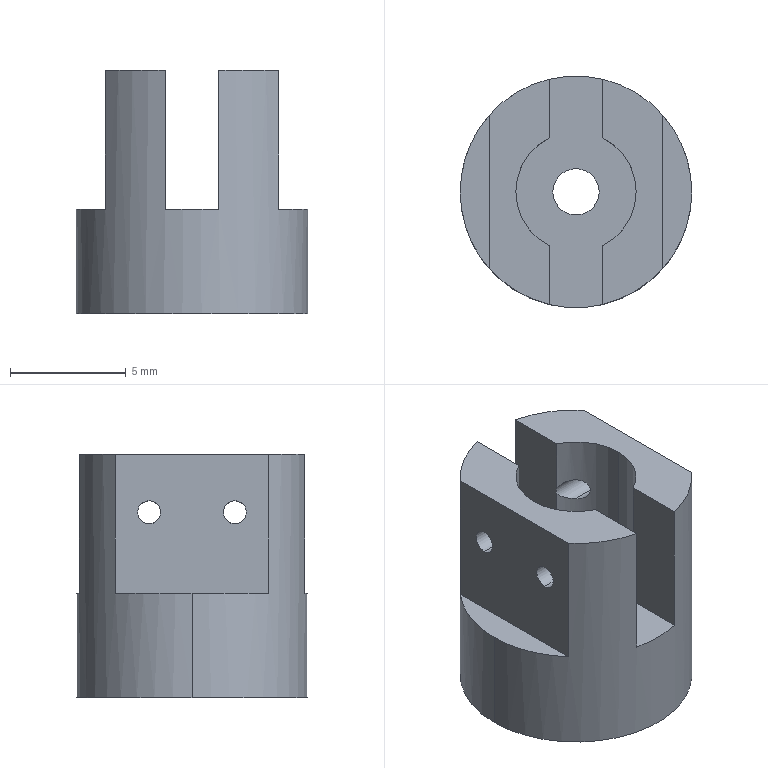Part | SolidWorks | features ICE 6, Extrusion 1 | 1 solid | 30 faces | box 10 x 10 x 10.5 mm | volume 483.8 mm3 | cylinder 17 | plane 13 | commonest cylinder face diameters 1 x8 5.2 x3 2 x2 5 x2 10 x2
STEP:
#1=CARTESIAN_POINT('',(3.75,1.85,7.5));
#2=VERTEX_POINT('',#1);
#3=CARTESIAN_POINT('',(3.75,1.85,8.5));
#4=VERTEX_POINT('',#3);
#5=CARTESIAN_POINT('',(3.75,1.85,8.));
#6=DIRECTION('',(-1.,0.,0.));
#7=DIRECTION('',(0.,0.,1.));
#8=AXIS2_PLACEMENT_3D('',#5,#6,#7);
#9=CIRCLE('',#8,0.5);
#10=EDGE_CURVE('',#2,#4,#9,.T.);
#11=ORIENTED_EDGE('',*,*,#10,.F.);
#12=CARTESIAN_POINT('',(1.827,1.85,7.5));
#13=VERTEX_POINT('',#12);
#14=CARTESIAN_POINT('',(5.,1.85,7.5));
#15=DIRECTION('',(-1.,0.,0.));
#16=VECTOR('',#15,1000.);
#17=LINE('',#14,#16);
#18=EDGE_CURVE('',#2,#13,#17,.T.);
#19=ORIENTED_EDGE('',*,*,#18,.T.);
#20=CARTESIAN_POINT('',(1.827,1.85,8.5));
#21=VERTEX_POINT('',#20);
#22=CARTESIAN_POINT('',(1.827,1.85,8.5));
#23=CARTESIAN_POINT('',(1.934,1.744,8.5));
#24=CARTESIAN_POINT('',(2.032,1.626,8.466));
#25=CARTESIAN_POINT('',(2.142,1.475,8.338));
#26=CARTESIAN_POINT('',(2.171,1.431,8.282));
#27=CARTESIAN_POINT('',(2.211,1.368,8.152));
#28=CARTESIAN_POINT('',(2.222,1.35,8.077));
#29=CARTESIAN_POINT('',(2.222,1.35,7.926));
#30=CARTESIAN_POINT('',(2.212,1.368,7.85));
#31=CARTESIAN_POINT('',(2.172,1.43,7.719));
#32=CARTESIAN_POINT('',(2.142,1.475,7.663));
#33=CARTESIAN_POINT('',(2.069,1.576,7.577));
#34=CARTESIAN_POINT('',(2.026,1.631,7.547));
#35=CARTESIAN_POINT('',(1.931,1.742,7.508));
#36=CARTESIAN_POINT('',(1.881,1.797,7.5));
#37=CARTESIAN_POINT('',(1.827,1.85,7.5));
#38=B_SPLINE_CURVE_WITH_KNOTS('',3,(#22,#23,#24,#25,#26,#27,#28,#29,#30,#31,#32,#33,#34,#35,#36,#37),.UNSPECIFIED.,.F.,.F.,(4,2,2,2,2,2,2,4),(0.0009388,0.001388,0.001612,0.001836,0.002061,0.002285,0.00251,0.002734),.UNSPECIFIED.);
#39=EDGE_CURVE('',#21,#13,#38,.T.);
#40=ORIENTED_EDGE('',*,*,#39,.F.);
#41=CARTESIAN_POINT('',(5.,1.85,8.5));
#42=DIRECTION('',(-1.,0.,0.));
#43=VECTOR('',#42,1000.);
#44=LINE('',#41,#43);
#45=EDGE_CURVE('',#4,#21,#44,.T.);
#46=ORIENTED_EDGE('',*,*,#45,.F.);
#47=EDGE_LOOP('',(#11,#19,#40,#46));
#48=FACE_OUTER_BOUND('',#47,.T.);
#49=CARTESIAN_POINT('',(5.,1.85,8.));
#50=DIRECTION('',(-1.,0.,0.));
#51=DIRECTION('',(0.,0.,1.));
#52=AXIS2_PLACEMENT_3D('',#49,#50,#51);
#53=CYLINDRICAL_SURFACE('',#52,0.5);
#54=ADVANCED_FACE('',(#48),#53,.F.);
#55=CARTESIAN_POINT('',(3.75,-1.85,7.5));
#56=VERTEX_POINT('',#55);
#57=CARTESIAN_POINT('',(3.75,-1.85,8.5));
#58=VERTEX_POINT('',#57);
#59=CARTESIAN_POINT('',(3.75,-1.85,8.));
#60=DIRECTION('',(-1.,0.,0.));
#61=DIRECTION('',(0.,0.,1.));
#62=AXIS2_PLACEMENT_3D('',#59,#60,#61);
#63=CIRCLE('',#62,0.5);
#64=EDGE_CURVE('',#56,#58,#63,.T.);
#65=ORIENTED_EDGE('',*,*,#64,.F.);
#66=CARTESIAN_POINT('',(1.827,-1.85,7.5));
#67=VERTEX_POINT('',#66);
#68=CARTESIAN_POINT('',(5.,-1.85,7.5));
#69=DIRECTION('',(-1.,0.,0.));
#70=VECTOR('',#69,1000.);
#71=LINE('',#68,#70);
#72=EDGE_CURVE('',#56,#67,#71,.T.);
#73=ORIENTED_EDGE('',*,*,#72,.T.);
#74=CARTESIAN_POINT('',(1.15,-2.332,7.866));
#75=VERTEX_POINT('',#74);
#76=CARTESIAN_POINT('',(1.15,-2.332,7.866));
#77=CARTESIAN_POINT('',(1.188,-2.313,7.799));
#78=CARTESIAN_POINT('',(1.242,-2.285,7.747));
#79=CARTESIAN_POINT('',(1.355,-2.22,7.659));
#80=CARTESIAN_POINT('',(1.414,-2.183,7.624));
#81=CARTESIAN_POINT('',(1.594,-2.059,7.535));
#82=CARTESIAN_POINT('',(1.715,-1.96,7.5));
#83=CARTESIAN_POINT('',(1.827,-1.85,7.5));
#84=B_SPLINE_CURVE_WITH_KNOTS('',3,(#76,#77,#78,#79,#80,#81,#82,#83),.UNSPECIFIED.,.F.,.F.,(4,2,2,4),(0.,0.0002347,0.0004694,0.0009388),.UNSPECIFIED.);
#85=EDGE_CURVE('',#75,#67,#84,.T.);
#86=ORIENTED_EDGE('',*,*,#85,.F.);
#87=CARTESIAN_POINT('',(1.15,-2.332,8.134));
#88=VERTEX_POINT('',#87);
#89=CARTESIAN_POINT('',(1.15,-1.85,8.));
#90=DIRECTION('',(1.,0.,0.));
#91=DIRECTION('',(0.,0.,-1.));
#92=AXIS2_PLACEMENT_3D('',#89,#90,#91);
#93=CIRCLE('',#92,0.5);
#94=EDGE_CURVE('',#88,#75,#93,.T.);
#95=ORIENTED_EDGE('',*,*,#94,.F.);
#96=CARTESIAN_POINT('',(1.827,-1.85,8.5));
#97=VERTEX_POINT('',#96);
#98=CARTESIAN_POINT('',(1.827,-1.85,8.5));
#99=CARTESIAN_POINT('',(1.714,-1.961,8.5));
#100=CARTESIAN_POINT('',(1.593,-2.06,8.465));
#101=CARTESIAN_POINT('',(1.414,-2.183,8.376));
#102=CARTESIAN_POINT('',(1.355,-2.22,8.341));
#103=CARTESIAN_POINT('',(1.242,-2.285,8.253));
#104=CARTESIAN_POINT('',(1.188,-2.313,8.201));
#105=CARTESIAN_POINT('',(1.15,-2.332,8.134));
#106=B_SPLINE_CURVE_WITH_KNOTS('',3,(#98,#99,#100,#101,#102,#103,#104,#105),.UNSPECIFIED.,.F.,.F.,(4,2,2,4),(0.002734,0.003203,0.003438,0.003673),.UNSPECIFIED.);
#107=EDGE_CURVE('',#97,#88,#106,.T.);
#108=ORIENTED_EDGE('',*,*,#107,.F.);
#109=CARTESIAN_POINT('',(5.,-1.85,8.5));
#110=DIRECTION('',(-1.,0.,0.));
#111=VECTOR('',#110,1000.);
#112=LINE('',#109,#111);
#113=EDGE_CURVE('',#58,#97,#112,.T.);
#114=ORIENTED_EDGE('',*,*,#113,.F.);
#115=EDGE_LOOP('',(#65,#73,#86,#95,#108,#114));
#116=FACE_OUTER_BOUND('',#115,.T.);
#117=CARTESIAN_POINT('',(5.,-1.85,8.));
#118=DIRECTION('',(-1.,0.,0.));
#119=DIRECTION('',(0.,0.,1.));
#120=AXIS2_PLACEMENT_3D('',#117,#118,#119);
#121=CYLINDRICAL_SURFACE('',#120,0.5);
#122=ADVANCED_FACE('',(#116),#121,.F.);
#123=CARTESIAN_POINT('',(-1.827,1.85,7.5));
#124=VERTEX_POINT('',#123);
#125=CARTESIAN_POINT('',(-1.827,1.85,8.5));
#126=VERTEX_POINT('',#125);
#127=CARTESIAN_POINT('',(-1.827,1.85,7.5));
#128=CARTESIAN_POINT('',(-1.934,1.744,7.5));
#129=CARTESIAN_POINT('',(-2.032,1.626,7.534));
#130=CARTESIAN_POINT('',(-2.142,1.475,7.662));
#131=CARTESIAN_POINT('',(-2.171,1.431,7.718));
#132=CARTESIAN_POINT('',(-2.211,1.368,7.848));
#133=CARTESIAN_POINT('',(-2.222,1.35,7.923));
#134=CARTESIAN_POINT('',(-2.222,1.35,8.074));
#135=CARTESIAN_POINT('',(-2.212,1.368,8.15));
#136=CARTESIAN_POINT('',(-2.172,1.43,8.281));
#137=CARTESIAN_POINT('',(-2.142,1.475,8.337));
#138=CARTESIAN_POINT('',(-2.069,1.576,8.423));
#139=CARTESIAN_POINT('',(-2.026,1.631,8.453));
#140=CARTESIAN_POINT('',(-1.931,1.742,8.492));
#141=CARTESIAN_POINT('',(-1.881,1.797,8.5));
#142=CARTESIAN_POINT('',(-1.827,1.85,8.5));
#143=B_SPLINE_CURVE_WITH_KNOTS('',3,(#127,#128,#129,#130,#131,#132,#133,#134,#135,#136,#137,#138,#139,#140,#141,#142),.UNSPECIFIED.,.F.,.F.,(4,2,2,2,2,2,2,4),(0.0009388,0.001388,0.001612,0.001836,0.002061,0.002285,0.00251,0.002734),.UNSPECIFIED.);
#144=EDGE_CURVE('',#124,#126,#143,.T.);
#145=ORIENTED_EDGE('',*,*,#144,.F.);
#146=CARTESIAN_POINT('',(-3.75,1.85,7.5));
#147=VERTEX_POINT('',#146);
#148=CARTESIAN_POINT('',(5.,1.85,7.5));
#149=DIRECTION('',(-1.,0.,0.));
#150=VECTOR('',#149,1000.);
#151=LINE('',#148,#150);
#152=EDGE_CURVE('',#124,#147,#151,.T.);
#153=ORIENTED_EDGE('',*,*,#152,.T.);
#154=CARTESIAN_POINT('',(-3.75,1.85,8.5));
#155=VERTEX_POINT('',#154);
#156=CARTESIAN_POINT('',(-3.75,1.85,8.));
#157=DIRECTION('',(-1.,0.,0.));
#158=DIRECTION('',(0.,0.,1.));
#159=AXIS2_PLACEMENT_3D('',#156,#157,#158);
#160=CIRCLE('',#159,0.5);
#161=EDGE_CURVE('',#147,#155,#160,.T.);
#162=ORIENTED_EDGE('',*,*,#161,.T.);
#163=CARTESIAN_POINT('',(5.,1.85,8.5));
#164=DIRECTION('',(-1.,0.,0.));
#165=VECTOR('',#164,1000.);
#166=LINE('',#163,#165);
#167=EDGE_CURVE('',#126,#155,#166,.T.);
#168=ORIENTED_EDGE('',*,*,#167,.F.);
#169=EDGE_LOOP('',(#145,#153,#162,#168));
#170=FACE_OUTER_BOUND('',#169,.T.);
#171=CARTESIAN_POINT('',(5.,1.85,8.));
#172=DIRECTION('',(-1.,0.,0.));
#173=DIRECTION('',(0.,0.,1.));
#174=AXIS2_PLACEMENT_3D('',#171,#172,#173);
#175=CYLINDRICAL_SURFACE('',#174,0.5);
#176=ADVANCED_FACE('',(#170),#175,.F.);
#177=CARTESIAN_POINT('',(-1.827,-1.85,7.5));
#178=VERTEX_POINT('',#177);
#179=CARTESIAN_POINT('',(-1.15,-2.332,7.866));
#180=VERTEX_POINT('',#179);
#181=CARTESIAN_POINT('',(-1.827,-1.85,7.5));
#182=CARTESIAN_POINT('',(-1.714,-1.961,7.5));
#183=CARTESIAN_POINT('',(-1.593,-2.06,7.535));
#184=CARTESIAN_POINT('',(-1.414,-2.183,7.624));
#185=CARTESIAN_POINT('',(-1.355,-2.22,7.659));
#186=CARTESIAN_POINT('',(-1.242,-2.285,7.747));
#187=CARTESIAN_POINT('',(-1.188,-2.313,7.799));
#188=CARTESIAN_POINT('',(-1.15,-2.332,7.866));
#189=B_SPLINE_CURVE_WITH_KNOTS('',3,(#181,#182,#183,#184,#185,#186,#187,#188),.UNSPECIFIED.,.F.,.F.,(4,2,2,4),(0.002734,0.003203,0.003438,0.003673),.UNSPECIFIED.);
#190=EDGE_CURVE('',#178,#180,#189,.T.);
#191=ORIENTED_EDGE('',*,*,#190,.F.);
#192=CARTESIAN_POINT('',(-3.75,-1.85,7.5));
#193=VERTEX_POINT('',#192);
#194=CARTESIAN_POINT('',(5.,-1.85,7.5));
#195=DIRECTION('',(-1.,0.,0.));
#196=VECTOR('',#195,1000.);
#197=LINE('',#194,#196);
#198=EDGE_CURVE('',#178,#193,#197,.T.);
#199=ORIENTED_EDGE('',*,*,#198,.T.);
#200=CARTESIAN_POINT('',(-3.75,-1.85,8.5));
#201=VERTEX_POINT('',#200);
#202=CARTESIAN_POINT('',(-3.75,-1.85,8.));
#203=DIRECTION('',(-1.,0.,0.));
#204=DIRECTION('',(0.,0.,1.));
#205=AXIS2_PLACEMENT_3D('',#202,#203,#204);
#206=CIRCLE('',#205,0.5);
#207=EDGE_CURVE('',#193,#201,#206,.T.);
#208=ORIENTED_EDGE('',*,*,#207,.T.);
#209=CARTESIAN_POINT('',(-1.827,-1.85,8.5));
#210=VERTEX_POINT('',#209);
#211=CARTESIAN_POINT('',(5.,-1.85,8.5));
#212=DIRECTION('',(-1.,0.,0.));
#213=VECTOR('',#212,1000.);
#214=LINE('',#211,#213);
#215=EDGE_CURVE('',#210,#201,#214,.T.);
#216=ORIENTED_EDGE('',*,*,#215,.F.);
#217=CARTESIAN_POINT('',(-1.15,-2.332,8.134));
#218=VERTEX_POINT('',#217);
#219=CARTESIAN_POINT('',(-1.15,-2.332,8.134));
#220=CARTESIAN_POINT('',(-1.188,-2.313,8.201));
#221=CARTESIAN_POINT('',(-1.242,-2.285,8.253));
#222=CARTESIAN_POINT('',(-1.355,-2.22,8.341));
#223=CARTESIAN_POINT('',(-1.414,-2.183,8.376));
#224=CARTESIAN_POINT('',(-1.594,-2.059,8.465));
#225=CARTESIAN_POINT('',(-1.715,-1.96,8.5));
#226=CARTESIAN_POINT('',(-1.827,-1.85,8.5));
#227=B_SPLINE_CURVE_WITH_KNOTS('',3,(#219,#220,#221,#222,#223,#224,#225,#226),.UNSPECIFIED.,.F.,.F.,(4,2,2,4),(0.,0.0002347,0.0004694,0.0009388),.UNSPECIFIED.);
#228=EDGE_CURVE('',#218,#210,#227,.T.);
#229=ORIENTED_EDGE('',*,*,#228,.F.);
#230=CARTESIAN_POINT('',(-1.15,-1.85,8.));
#231=DIRECTION('',(-1.,0.,0.));
#232=DIRECTION('',(0.,0.,1.));
#233=AXIS2_PLACEMENT_3D('',#230,#231,#232);
#234=CIRCLE('',#233,0.5);
#235=EDGE_CURVE('',#180,#218,#234,.T.);
#236=ORIENTED_EDGE('',*,*,#235,.F.);
#237=EDGE_LOOP('',(#191,#199,#208,#216,#229,#236));
#238=FACE_OUTER_BOUND('',#237,.T.);
#239=CARTESIAN_POINT('',(5.,-1.85,8.));
#240=DIRECTION('',(-1.,0.,0.));
#241=DIRECTION('',(0.,0.,1.));
#242=AXIS2_PLACEMENT_3D('',#239,#240,#241);
#243=CYLINDRICAL_SURFACE('',#242,0.5);
#244=ADVANCED_FACE('',(#238),#243,.F.);
#245=CARTESIAN_POINT('',(2.6,0.,4.5));
#246=VERTEX_POINT('',#245);
#247=CARTESIAN_POINT('',(1.15,2.332,4.5));
#248=VERTEX_POINT('',#247);
#249=CARTESIAN_POINT('',(0.,0.,4.5));
#250=DIRECTION('',(0.,0.,1.));
#251=DIRECTION('',(-1.,0.,0.));
#252=AXIS2_PLACEMENT_3D('',#249,#250,#251);
#253=CIRCLE('',#252,2.6);
#254=EDGE_CURVE('',#246,#248,#253,.T.);
#255=ORIENTED_EDGE('',*,*,#254,.F.);
#256=CARTESIAN_POINT('',(2.6,0.,10.5));
#257=VERTEX_POINT('',#256);
#258=CARTESIAN_POINT('',(2.6,0.,-2.854));
#259=DIRECTION('',(0.,0.,1.));
#260=VECTOR('',#259,1000.);
#261=LINE('',#258,#260);
#262=EDGE_CURVE('',#246,#257,#261,.T.);
#263=ORIENTED_EDGE('',*,*,#262,.T.);
#264=CARTESIAN_POINT('',(1.15,2.332,10.5));
#265=VERTEX_POINT('',#264);
#266=CARTESIAN_POINT('',(0.,0.,10.5));
#267=DIRECTION('',(0.,0.,1.));
#268=DIRECTION('',(1.,0.,0.));
#269=AXIS2_PLACEMENT_3D('',#266,#267,#268);
#270=CIRCLE('',#269,2.6);
#271=EDGE_CURVE('',#257,#265,#270,.T.);
#272=ORIENTED_EDGE('',*,*,#271,.T.);
#273=CARTESIAN_POINT('',(1.15,2.332,8.134));
#274=VERTEX_POINT('',#273);
#275=CARTESIAN_POINT('',(1.15,2.332,-2.854));
#276=DIRECTION('',(0.,0.,1.));
#277=VECTOR('',#276,1000.);
#278=LINE('',#275,#277);
#279=EDGE_CURVE('',#274,#265,#278,.T.);
#280=ORIENTED_EDGE('',*,*,#279,.F.);
#281=CARTESIAN_POINT('',(1.15,2.332,8.134));
#282=CARTESIAN_POINT('',(1.188,2.313,8.201));
#283=CARTESIAN_POINT('',(1.242,2.285,8.253));
#284=CARTESIAN_POINT('',(1.355,2.22,8.341));
#285=CARTESIAN_POINT('',(1.414,2.183,8.376));
#286=CARTESIAN_POINT('',(1.594,2.059,8.465));
#287=CARTESIAN_POINT('',(1.715,1.96,8.5));
#288=CARTESIAN_POINT('',(1.827,1.85,8.5));
#289=B_SPLINE_CURVE_WITH_KNOTS('',3,(#281,#282,#283,#284,#285,#286,#287,#288),.UNSPECIFIED.,.F.,.F.,(4,2,2,4),(0.,0.0002347,0.0004694,0.0009388),.UNSPECIFIED.);
#290=EDGE_CURVE('',#274,#21,#289,.T.);
#291=ORIENTED_EDGE('',*,*,#290,.T.);
#292=ORIENTED_EDGE('',*,*,#39,.T.);
#293=CARTESIAN_POINT('',(1.15,2.332,7.866));
#294=VERTEX_POINT('',#293);
#295=CARTESIAN_POINT('',(1.827,1.85,7.5));
#296=CARTESIAN_POINT('',(1.714,1.961,7.5));
#297=CARTESIAN_POINT('',(1.593,2.06,7.535));
#298=CARTESIAN_POINT('',(1.414,2.183,7.624));
#299=CARTESIAN_POINT('',(1.355,2.22,7.659));
#300=CARTESIAN_POINT('',(1.242,2.285,7.747));
#301=CARTESIAN_POINT('',(1.188,2.313,7.799));
#302=CARTESIAN_POINT('',(1.15,2.332,7.866));
#303=B_SPLINE_CURVE_WITH_KNOTS('',3,(#295,#296,#297,#298,#299,#300,#301,#302),.UNSPECIFIED.,.F.,.F.,(4,2,2,4),(0.002734,0.003203,0.003438,0.003673),.UNSPECIFIED.);
#304=EDGE_CURVE('',#13,#294,#303,.T.);
#305=ORIENTED_EDGE('',*,*,#304,.T.);
#306=CARTESIAN_POINT('',(1.15,2.332,-2.854));
#307=DIRECTION('',(0.,0.,1.));
#308=VECTOR('',#307,1000.);
#309=LINE('',#306,#308);
#310=EDGE_CURVE('',#248,#294,#309,.T.);
#311=ORIENTED_EDGE('',*,*,#310,.F.);
#312=EDGE_LOOP('',(#255,#263,#272,#280,#291,#292,#305,#311));
#313=FACE_OUTER_BOUND('',#312,.T.);
#314=CARTESIAN_POINT('',(0.,0.,-2.854));
#315=DIRECTION('',(0.,0.,1.));
#316=DIRECTION('',(1.,0.,0.));
#317=AXIS2_PLACEMENT_3D('',#314,#315,#316);
#318=CYLINDRICAL_SURFACE('',#317,2.6);
#319=ADVANCED_FACE('',(#313),#318,.F.);
#320=CARTESIAN_POINT('',(-1.,0.,4.5));
#321=VERTEX_POINT('',#320);
#322=CARTESIAN_POINT('',(1.,0.,4.5));
#323=VERTEX_POINT('',#322);
#324=CARTESIAN_POINT('',(0.,0.,4.5));
#325=DIRECTION('',(0.,0.,1.));
#326=DIRECTION('',(-1.,0.,0.));
#327=AXIS2_PLACEMENT_3D('',#324,#325,#326);
#328=CIRCLE('',#327,1.);
#329=EDGE_CURVE('',#321,#323,#328,.T.);
#330=ORIENTED_EDGE('',*,*,#329,.T.);
#331=CARTESIAN_POINT('',(1.,0.,3.5));
#332=VERTEX_POINT('',#331);
#333=CARTESIAN_POINT('',(1.,0.,10.5));
#334=DIRECTION('',(0.,0.,-1.));
#335=VECTOR('',#334,1000.);
#336=LINE('',#333,#335);
#337=EDGE_CURVE('',#323,#332,#336,.T.);
#338=ORIENTED_EDGE('',*,*,#337,.T.);
#339=CARTESIAN_POINT('',(-1.,0.,3.5));
#340=VERTEX_POINT('',#339);
#341=CARTESIAN_POINT('',(0.,0.,3.5));
#342=DIRECTION('',(0.,0.,-1.));
#343=DIRECTION('',(-1.,0.,0.));
#344=AXIS2_PLACEMENT_3D('',#341,#342,#343);
#345=CIRCLE('',#344,1.);
#346=EDGE_CURVE('',#332,#340,#345,.T.);
#347=ORIENTED_EDGE('',*,*,#346,.T.);
#348=CARTESIAN_POINT('',(-1.,0.,10.5));
#349=DIRECTION('',(0.,0.,-1.));
#350=VECTOR('',#349,1000.);
#351=LINE('',#348,#350);
#352=EDGE_CURVE('',#321,#340,#351,.T.);
#353=ORIENTED_EDGE('',*,*,#352,.F.);
#354=EDGE_LOOP('',(#330,#338,#347,#353));
#355=FACE_OUTER_BOUND('',#354,.T.);
#356=CARTESIAN_POINT('',(0.,0.,10.5));
#357=DIRECTION('',(0.,0.,-1.));
#358=DIRECTION('',(-1.,0.,0.));
#359=AXIS2_PLACEMENT_3D('',#356,#357,#358);
#360=CYLINDRICAL_SURFACE('',#359,1.);
#361=ADVANCED_FACE('',(#355),#360,.F.);
#362=CARTESIAN_POINT('',(2.5,0.,3.5));
#363=VERTEX_POINT('',#362);
#364=CARTESIAN_POINT('',(-2.5,0.,3.5));
#365=VERTEX_POINT('',#364);
#366=CARTESIAN_POINT('',(0.,0.,3.5));
#367=DIRECTION('',(0.,0.,-1.));
#368=DIRECTION('',(-1.,0.,0.));
#369=AXIS2_PLACEMENT_3D('',#366,#367,#368);
#370=CIRCLE('',#369,2.5);
#371=EDGE_CURVE('',#363,#365,#370,.T.);
#372=ORIENTED_EDGE('',*,*,#371,.F.);
#373=CARTESIAN_POINT('',(2.5,0.,0.));
#374=VERTEX_POINT('',#373);
#375=CARTESIAN_POINT('',(2.5,0.,3.5));
#376=DIRECTION('',(0.,0.,-1.));
#377=VECTOR('',#376,1000.);
#378=LINE('',#375,#377);
#379=EDGE_CURVE('',#363,#374,#378,.T.);
#380=ORIENTED_EDGE('',*,*,#379,.T.);
#381=CARTESIAN_POINT('',(-2.5,0.,0.));
#382=VERTEX_POINT('',#381);
#383=CARTESIAN_POINT('',(0.,0.,0.));
#384=DIRECTION('',(0.,0.,-1.));
#385=DIRECTION('',(-1.,0.,0.));
#386=AXIS2_PLACEMENT_3D('',#383,#384,#385);
#387=CIRCLE('',#386,2.5);
#388=EDGE_CURVE('',#374,#382,#387,.T.);
#389=ORIENTED_EDGE('',*,*,#388,.T.);
#390=CARTESIAN_POINT('',(-2.5,0.,3.5));
#391=DIRECTION('',(0.,0.,-1.));
#392=VECTOR('',#391,1000.);
#393=LINE('',#390,#392);
#394=EDGE_CURVE('',#365,#382,#393,.T.);
#395=ORIENTED_EDGE('',*,*,#394,.F.);
#396=EDGE_LOOP('',(#372,#380,#389,#395));
#397=FACE_OUTER_BOUND('',#396,.T.);
#398=CARTESIAN_POINT('',(0.,0.,3.5));
#399=DIRECTION('',(0.,0.,-1.));
#400=DIRECTION('',(-1.,0.,0.));
#401=AXIS2_PLACEMENT_3D('',#398,#399,#400);
#402=CYLINDRICAL_SURFACE('',#401,2.5);
#403=ADVANCED_FACE('',(#397),#402,.F.);
#404=CARTESIAN_POINT('',(3.75,3.307,4.5));
#405=VERTEX_POINT('',#404);
#406=CARTESIAN_POINT('',(5.,0.,4.5));
#407=VERTEX_POINT('',#406);
#408=CARTESIAN_POINT('',(0.,0.,4.5));
#409=DIRECTION('',(0.,0.,-1.));
#410=DIRECTION('',(-1.,0.,0.));
#411=AXIS2_PLACEMENT_3D('',#408,#409,#410);
#412=CIRCLE('',#411,5.);
#413=EDGE_CURVE('',#405,#407,#412,.T.);
#414=ORIENTED_EDGE('',*,*,#413,.T.);
#415=CARTESIAN_POINT('',(5.,0.,0.));
#416=VERTEX_POINT('',#415);
#417=CARTESIAN_POINT('',(5.,0.,10.5));
#418=DIRECTION('',(0.,0.,-1.));
#419=VECTOR('',#418,1000.);
#420=LINE('',#417,#419);
#421=EDGE_CURVE('',#407,#416,#420,.T.);
#422=ORIENTED_EDGE('',*,*,#421,.T.);
#423=CARTESIAN_POINT('',(-5.,0.,0.));
#424=VERTEX_POINT('',#423);
#425=CARTESIAN_POINT('',(0.,0.,0.));
#426=DIRECTION('',(0.,0.,1.));
#427=DIRECTION('',(1.,0.,0.));
#428=AXIS2_PLACEMENT_3D('',#425,#426,#427);
#429=CIRCLE('',#428,5.);
#430=EDGE_CURVE('',#416,#424,#429,.T.);
#431=ORIENTED_EDGE('',*,*,#430,.T.);
#432=CARTESIAN_POINT('',(-5.,0.,4.5));
#433=VERTEX_POINT('',#432);
#434=CARTESIAN_POINT('',(-5.,0.,10.5));
#435=DIRECTION('',(0.,0.,-1.));
#436=VECTOR('',#435,1000.);
#437=LINE('',#434,#436);
#438=EDGE_CURVE('',#433,#424,#437,.T.);
#439=ORIENTED_EDGE('',*,*,#438,.F.);
#440=CARTESIAN_POINT('',(-3.75,3.307,4.5));
#441=VERTEX_POINT('',#440);
#442=CARTESIAN_POINT('',(0.,0.,4.5));
#443=DIRECTION('',(0.,0.,-1.));
#444=DIRECTION('',(-1.,0.,0.));
#445=AXIS2_PLACEMENT_3D('',#442,#443,#444);
#446=CIRCLE('',#445,5.);
#447=EDGE_CURVE('',#433,#441,#446,.T.);
#448=ORIENTED_EDGE('',*,*,#447,.T.);
#449=CARTESIAN_POINT('',(-3.75,3.307,10.5));
#450=VERTEX_POINT('',#449);
#451=CARTESIAN_POINT('',(-3.75,3.307,10.5));
#452=DIRECTION('',(0.,0.,1.));
#453=VECTOR('',#452,1000.);
#454=LINE('',#451,#453);
#455=EDGE_CURVE('',#441,#450,#454,.T.);
#456=ORIENTED_EDGE('',*,*,#455,.T.);
#457=CARTESIAN_POINT('',(-1.15,4.866,10.5));
#458=VERTEX_POINT('',#457);
#459=CARTESIAN_POINT('',(0.,0.,10.5));
#460=DIRECTION('',(0.,0.,1.));
#461=DIRECTION('',(1.,0.,0.));
#462=AXIS2_PLACEMENT_3D('',#459,#460,#461);
#463=CIRCLE('',#462,5.);
#464=EDGE_CURVE('',#458,#450,#463,.T.);
#465=ORIENTED_EDGE('',*,*,#464,.F.);
#466=CARTESIAN_POINT('',(-1.15,4.866,4.5));
#467=VERTEX_POINT('',#466);
#468=CARTESIAN_POINT('',(-1.15,4.866,10.5));
#469=DIRECTION('',(0.,0.,-1.));
#470=VECTOR('',#469,1000.);
#471=LINE('',#468,#470);
#472=EDGE_CURVE('',#458,#467,#471,.T.);
#473=ORIENTED_EDGE('',*,*,#472,.T.);
#474=CARTESIAN_POINT('',(1.15,4.866,4.5));
#475=VERTEX_POINT('',#474);
#476=CARTESIAN_POINT('',(0.,0.,4.5));
#477=DIRECTION('',(0.,0.,-1.));
#478=DIRECTION('',(-1.,0.,0.));
#479=AXIS2_PLACEMENT_3D('',#476,#477,#478);
#480=CIRCLE('',#479,5.);
#481=EDGE_CURVE('',#467,#475,#480,.T.);
#482=ORIENTED_EDGE('',*,*,#481,.T.);
#483=CARTESIAN_POINT('',(1.15,4.866,10.5));
#484=VERTEX_POINT('',#483);
#485=CARTESIAN_POINT('',(1.15,4.866,10.5));
#486=DIRECTION('',(0.,0.,1.));
#487=VECTOR('',#486,1000.);
#488=LINE('',#485,#487);
#489=EDGE_CURVE('',#475,#484,#488,.T.);
#490=ORIENTED_EDGE('',*,*,#489,.T.);
#491=CARTESIAN_POINT('',(3.75,3.307,10.5));
#492=VERTEX_POINT('',#491);
#493=CARTESIAN_POINT('',(0.,0.,10.5));
#494=DIRECTION('',(0.,0.,1.));
#495=DIRECTION('',(1.,0.,0.));
#496=AXIS2_PLACEMENT_3D('',#493,#494,#495);
#497=CIRCLE('',#496,5.);
#498=EDGE_CURVE('',#492,#484,#497,.T.);
#499=ORIENTED_EDGE('',*,*,#498,.F.);
#500=CARTESIAN_POINT('',(3.75,3.307,10.5));
#501=DIRECTION('',(0.,0.,-1.));
#502=VECTOR('',#501,1000.);
#503=LINE('',#500,#502);
#504=EDGE_CURVE('',#492,#405,#503,.T.);
#505=ORIENTED_EDGE('',*,*,#504,.T.);
#506=EDGE_LOOP('',(#414,#422,#431,#439,#448,#456,#465,#473,#482,#490,#499,#505));
#507=FACE_OUTER_BOUND('',#506,.T.);
#508=CARTESIAN_POINT('',(0.,0.,10.5));
#509=DIRECTION('',(0.,0.,-1.));
#510=DIRECTION('',(-1.,0.,0.));
#511=AXIS2_PLACEMENT_3D('',#508,#509,#510);
#512=CYLINDRICAL_SURFACE('',#511,5.);
#513=ADVANCED_FACE('',(#507),#512,.T.);
#514=CARTESIAN_POINT('',(-1.15,-2.332,4.5));
#515=VERTEX_POINT('',#514);
#516=CARTESIAN_POINT('',(-1.15,-2.332,-2.854));
#517=DIRECTION('',(0.,0.,1.));
#518=VECTOR('',#517,1000.);
#519=LINE('',#516,#518);
#520=EDGE_CURVE('',#515,#180,#519,.T.);
#521=ORIENTED_EDGE('',*,*,#520,.T.);
#522=ORIENTED_EDGE('',*,*,#235,.T.);
#523=CARTESIAN_POINT('',(-1.15,-2.332,10.5));
#524=VERTEX_POINT('',#523);
#525=CARTESIAN_POINT('',(-1.15,-2.332,-2.854));
#526=DIRECTION('',(0.,0.,1.));
#527=VECTOR('',#526,1000.);
#528=LINE('',#525,#527);
#529=EDGE_CURVE('',#218,#524,#528,.T.);
#530=ORIENTED_EDGE('',*,*,#529,.T.);
#531=CARTESIAN_POINT('',(-1.15,-4.866,10.5));
#532=VERTEX_POINT('',#531);
#533=CARTESIAN_POINT('',(-1.15,-5.,10.5));
#534=DIRECTION('',(0.,1.,0.));
#535=VECTOR('',#534,1000.);
#536=LINE('',#533,#535);
#537=EDGE_CURVE('',#532,#524,#536,.T.);
#538=ORIENTED_EDGE('',*,*,#537,.F.);
#539=CARTESIAN_POINT('',(-1.15,-4.866,4.5));
#540=VERTEX_POINT('',#539);
#541=CARTESIAN_POINT('',(-1.15,-4.866,10.5));
#542=DIRECTION('',(0.,0.,1.));
#543=VECTOR('',#542,1000.);
#544=LINE('',#541,#543);
#545=EDGE_CURVE('',#540,#532,#544,.T.);
#546=ORIENTED_EDGE('',*,*,#545,.F.);
#547=CARTESIAN_POINT('',(-1.15,-5.,4.5));
#548=DIRECTION('',(0.,1.,0.));
#549=VECTOR('',#548,1000.);
#550=LINE('',#547,#549);
#551=EDGE_CURVE('',#540,#515,#550,.T.);
#552=ORIENTED_EDGE('',*,*,#551,.T.);
#553=EDGE_LOOP('',(#521,#522,#530,#538,#546,#552));
#554=FACE_OUTER_BOUND('',#553,.T.);
#555=CARTESIAN_POINT('',(-1.15,-5.,10.5));
#556=DIRECTION('',(-1.,0.,0.));
#557=DIRECTION('',(0.,0.,1.));
#558=AXIS2_PLACEMENT_3D('',#555,#556,#557);
#559=PLANE('',#558);
#560=ADVANCED_FACE('',(#554),#559,.F.);
#561=ORIENTED_EDGE('',*,*,#310,.T.);
#562=CARTESIAN_POINT('',(1.15,1.85,8.));
#563=DIRECTION('',(1.,0.,0.));
#564=DIRECTION('',(0.,0.,-1.));
#565=AXIS2_PLACEMENT_3D('',#562,#563,#564);
#566=CIRCLE('',#565,0.5);
#567=EDGE_CURVE('',#294,#274,#566,.T.);
#568=ORIENTED_EDGE('',*,*,#567,.T.);
#569=ORIENTED_EDGE('',*,*,#279,.T.);
#570=CARTESIAN_POINT('',(1.15,-5.,10.5));
#571=DIRECTION('',(0.,1.,0.));
#572=VECTOR('',#571,1000.);
#573=LINE('',#570,#572);
#574=EDGE_CURVE('',#265,#484,#573,.T.);
#575=ORIENTED_EDGE('',*,*,#574,.T.);
#576=ORIENTED_EDGE('',*,*,#489,.F.);
#577=CARTESIAN_POINT('',(1.15,-5.,4.5));
#578=DIRECTION('',(0.,1.,0.));
#579=VECTOR('',#578,1000.);
#580=LINE('',#577,#579);
#581=EDGE_CURVE('',#248,#475,#580,.T.);
#582=ORIENTED_EDGE('',*,*,#581,.F.);
#583=EDGE_LOOP('',(#561,#568,#569,#575,#576,#582));
#584=FACE_OUTER_BOUND('',#583,.T.);
#585=CARTESIAN_POINT('',(1.15,-5.,10.5));
#586=DIRECTION('',(1.,0.,0.));
#587=DIRECTION('',(0.,0.,-1.));
#588=AXIS2_PLACEMENT_3D('',#585,#586,#587);
#589=PLANE('',#588);
#590=ADVANCED_FACE('',(#584),#589,.F.);
#591=CARTESIAN_POINT('',(-1.15,2.332,10.5));
#592=VERTEX_POINT('',#591);
#593=CARTESIAN_POINT('',(0.,0.,10.5));
#594=DIRECTION('',(0.,0.,1.));
#595=DIRECTION('',(1.,0.,0.));
#596=AXIS2_PLACEMENT_3D('',#593,#594,#595);
#597=CIRCLE('',#596,2.6);
#598=EDGE_CURVE('',#592,#524,#597,.T.);
#599=ORIENTED_EDGE('',*,*,#598,.F.);
#600=CARTESIAN_POINT('',(-1.15,-5.,10.5));
#601=DIRECTION('',(0.,1.,0.));
#602=VECTOR('',#601,1000.);
#603=LINE('',#600,#602);
#604=EDGE_CURVE('',#592,#458,#603,.T.);
#605=ORIENTED_EDGE('',*,*,#604,.T.);
#606=ORIENTED_EDGE('',*,*,#464,.T.);
#607=CARTESIAN_POINT('',(-3.75,-3.307,10.5));
#608=VERTEX_POINT('',#607);
#609=CARTESIAN_POINT('',(-3.75,0.,10.5));
#610=DIRECTION('',(0.,1.,0.));
#611=VECTOR('',#610,1000.);
#612=LINE('',#609,#611);
#613=EDGE_CURVE('',#608,#450,#612,.T.);
#614=ORIENTED_EDGE('',*,*,#613,.F.);
#615=CARTESIAN_POINT('',(0.,0.,10.5));
#616=DIRECTION('',(0.,0.,1.));
#617=DIRECTION('',(1.,0.,0.));
#618=AXIS2_PLACEMENT_3D('',#615,#616,#617);
#619=CIRCLE('',#618,5.);
#620=EDGE_CURVE('',#608,#532,#619,.T.);
#621=ORIENTED_EDGE('',*,*,#620,.T.);
#622=ORIENTED_EDGE('',*,*,#537,.T.);
#623=EDGE_LOOP('',(#599,#605,#606,#614,#621,#622));
#624=FACE_OUTER_BOUND('',#623,.T.);
#625=CARTESIAN_POINT('',(0.,0.,10.5));
#626=DIRECTION('',(0.,0.,1.));
#627=DIRECTION('',(1.,0.,0.));
#628=AXIS2_PLACEMENT_3D('',#625,#626,#627);
#629=PLANE('',#628);
#630=ADVANCED_FACE('',(#624),#629,.T.);
#631=ORIENTED_EDGE('',*,*,#421,.F.);
#632=CARTESIAN_POINT('',(3.75,-3.307,4.5));
#633=VERTEX_POINT('',#632);
#634=CARTESIAN_POINT('',(0.,0.,4.5));
#635=DIRECTION('',(0.,0.,-1.));
#636=DIRECTION('',(-1.,0.,0.));
#637=AXIS2_PLACEMENT_3D('',#634,#635,#636);
#638=CIRCLE('',#637,5.);
#639=EDGE_CURVE('',#407,#633,#638,.T.);
#640=ORIENTED_EDGE('',*,*,#639,.T.);
#641=CARTESIAN_POINT('',(3.75,-3.307,10.5));
#642=VERTEX_POINT('',#641);
#643=CARTESIAN_POINT('',(3.75,-3.307,10.5));
#644=DIRECTION('',(0.,0.,1.));
#645=VECTOR('',#644,1000.);
#646=LINE('',#643,#645);
#647=EDGE_CURVE('',#633,#642,#646,.T.);
#648=ORIENTED_EDGE('',*,*,#647,.T.);
#649=CARTESIAN_POINT('',(1.15,-4.866,10.5));
#650=VERTEX_POINT('',#649);
#651=CARTESIAN_POINT('',(0.,0.,10.5));
#652=DIRECTION('',(0.,0.,1.));
#653=DIRECTION('',(1.,0.,0.));
#654=AXIS2_PLACEMENT_3D('',#651,#652,#653);
#655=CIRCLE('',#654,5.);
#656=EDGE_CURVE('',#650,#642,#655,.T.);
#657=ORIENTED_EDGE('',*,*,#656,.F.);
#658=CARTESIAN_POINT('',(1.15,-4.866,4.5));
#659=VERTEX_POINT('',#658);
#660=CARTESIAN_POINT('',(1.15,-4.866,10.5));
#661=DIRECTION('',(0.,0.,-1.));
#662=VECTOR('',#661,1000.);
#663=LINE('',#660,#662);
#664=EDGE_CURVE('',#650,#659,#663,.T.);
#665=ORIENTED_EDGE('',*,*,#664,.T.);
#666=CARTESIAN_POINT('',(0.,0.,4.5));
#667=DIRECTION('',(0.,0.,-1.));
#668=DIRECTION('',(-1.,0.,0.));
#669=AXIS2_PLACEMENT_3D('',#666,#667,#668);
#670=CIRCLE('',#669,5.);
#671=EDGE_CURVE('',#659,#540,#670,.T.);
#672=ORIENTED_EDGE('',*,*,#671,.T.);
#673=ORIENTED_EDGE('',*,*,#545,.T.);
#674=ORIENTED_EDGE('',*,*,#620,.F.);
#675=CARTESIAN_POINT('',(-3.75,-3.307,4.5));
#676=VERTEX_POINT('',#675);
#677=CARTESIAN_POINT('',(-3.75,-3.307,10.5));
#678=DIRECTION('',(0.,0.,-1.));
#679=VECTOR('',#678,1000.);
#680=LINE('',#677,#679);
#681=EDGE_CURVE('',#608,#676,#680,.T.);
#682=ORIENTED_EDGE('',*,*,#681,.T.);
#683=CARTESIAN_POINT('',(0.,0.,4.5));
#684=DIRECTION('',(0.,0.,-1.));
#685=DIRECTION('',(-1.,0.,0.));
#686=AXIS2_PLACEMENT_3D('',#683,#684,#685);
#687=CIRCLE('',#686,5.);
#688=EDGE_CURVE('',#676,#433,#687,.T.);
#689=ORIENTED_EDGE('',*,*,#688,.T.);
#690=ORIENTED_EDGE('',*,*,#438,.T.);
#691=CARTESIAN_POINT('',(0.,0.,0.));
#692=DIRECTION('',(0.,0.,1.));
#693=DIRECTION('',(1.,0.,0.));
#694=AXIS2_PLACEMENT_3D('',#691,#692,#693);
#695=CIRCLE('',#694,5.);
#696=EDGE_CURVE('',#424,#416,#695,.T.);
#697=ORIENTED_EDGE('',*,*,#696,.T.);
#698=EDGE_LOOP('',(#631,#640,#648,#657,#665,#672,#673,#674,#682,#689,#690,#697));
#699=FACE_OUTER_BOUND('',#698,.T.);
#700=CARTESIAN_POINT('',(0.,0.,10.5));
#701=DIRECTION('',(0.,0.,-1.));
#702=DIRECTION('',(-1.,0.,0.));
#703=AXIS2_PLACEMENT_3D('',#700,#701,#702);
#704=CYLINDRICAL_SURFACE('',#703,5.);
#705=ADVANCED_FACE('',(#699),#704,.T.);
#706=CARTESIAN_POINT('',(1.15,-2.332,10.5));
#707=VERTEX_POINT('',#706);
#708=CARTESIAN_POINT('',(0.,0.,10.5));
#709=DIRECTION('',(0.,0.,1.));
#710=DIRECTION('',(1.,0.,0.));
#711=AXIS2_PLACEMENT_3D('',#708,#709,#710);
#712=CIRCLE('',#711,2.6);
#713=EDGE_CURVE('',#707,#257,#712,.T.);
#714=ORIENTED_EDGE('',*,*,#713,.F.);
#715=CARTESIAN_POINT('',(1.15,-5.,10.5));
#716=DIRECTION('',(0.,1.,0.));
#717=VECTOR('',#716,1000.);
#718=LINE('',#715,#717);
#719=EDGE_CURVE('',#650,#707,#718,.T.);
#720=ORIENTED_EDGE('',*,*,#719,.F.);
#721=ORIENTED_EDGE('',*,*,#656,.T.);
#722=CARTESIAN_POINT('',(3.75,0.,10.5));
#723=DIRECTION('',(0.,-1.,0.));
#724=VECTOR('',#723,1000.);
#725=LINE('',#722,#724);
#726=EDGE_CURVE('',#492,#642,#725,.T.);
#727=ORIENTED_EDGE('',*,*,#726,.F.);
#728=ORIENTED_EDGE('',*,*,#498,.T.);
#729=ORIENTED_EDGE('',*,*,#574,.F.);
#730=ORIENTED_EDGE('',*,*,#271,.F.);
#731=EDGE_LOOP('',(#714,#720,#721,#727,#728,#729,#730));
#732=FACE_OUTER_BOUND('',#731,.T.);
#733=CARTESIAN_POINT('',(0.,0.,10.5));
#734=DIRECTION('',(0.,0.,1.));
#735=DIRECTION('',(1.,0.,0.));
#736=AXIS2_PLACEMENT_3D('',#733,#734,#735);
#737=PLANE('',#736);
#738=ADVANCED_FACE('',(#732),#737,.T.);
#739=CARTESIAN_POINT('',(0.,0.,0.));
#740=DIRECTION('',(0.,0.,-1.));
#741=DIRECTION('',(-1.,0.,0.));
#742=AXIS2_PLACEMENT_3D('',#739,#740,#741);
#743=CIRCLE('',#742,2.5);
#744=EDGE_CURVE('',#382,#374,#743,.T.);
#745=ORIENTED_EDGE('',*,*,#744,.F.);
#746=ORIENTED_EDGE('',*,*,#388,.F.);
#747=EDGE_LOOP('',(#745,#746));
#748=FACE_BOUND('',#747,.T.);
#749=ORIENTED_EDGE('',*,*,#696,.F.);
#750=ORIENTED_EDGE('',*,*,#430,.F.);
#751=EDGE_LOOP('',(#749,#750));
#752=FACE_OUTER_BOUND('',#751,.T.);
#753=CARTESIAN_POINT('',(0.,0.,0.));
#754=DIRECTION('',(0.,0.,1.));
#755=DIRECTION('',(1.,0.,0.));
#756=AXIS2_PLACEMENT_3D('',#753,#754,#755);
#757=PLANE('',#756);
#758=ADVANCED_FACE('',(#748,#752),#757,.F.);
#759=ORIENTED_EDGE('',*,*,#379,.F.);
#760=CARTESIAN_POINT('',(0.,0.,3.5));
#761=DIRECTION('',(0.,0.,-1.));
#762=DIRECTION('',(-1.,0.,0.));
#763=AXIS2_PLACEMENT_3D('',#760,#761,#762);
#764=CIRCLE('',#763,2.5);
#765=EDGE_CURVE('',#365,#363,#764,.T.);
#766=ORIENTED_EDGE('',*,*,#765,.F.);
#767=ORIENTED_EDGE('',*,*,#394,.T.);
#768=ORIENTED_EDGE('',*,*,#744,.T.);
#769=EDGE_LOOP('',(#759,#766,#767,#768));
#770=FACE_OUTER_BOUND('',#769,.T.);
#771=CARTESIAN_POINT('',(0.,0.,3.5));
#772=DIRECTION('',(0.,0.,-1.));
#773=DIRECTION('',(-1.,0.,0.));
#774=AXIS2_PLACEMENT_3D('',#771,#772,#773);
#775=CYLINDRICAL_SURFACE('',#774,2.5);
#776=ADVANCED_FACE('',(#770),#775,.F.);
#777=CARTESIAN_POINT('',(0.,0.,3.5));
#778=DIRECTION('',(0.,0.,-1.));
#779=DIRECTION('',(-1.,0.,0.));
#780=AXIS2_PLACEMENT_3D('',#777,#778,#779);
#781=CIRCLE('',#780,1.);
#782=EDGE_CURVE('',#340,#332,#781,.T.);
#783=ORIENTED_EDGE('',*,*,#782,.F.);
#784=ORIENTED_EDGE('',*,*,#346,.F.);
#785=EDGE_LOOP('',(#783,#784));
#786=FACE_BOUND('',#785,.T.);
#787=ORIENTED_EDGE('',*,*,#765,.T.);
#788=ORIENTED_EDGE('',*,*,#371,.T.);
#789=EDGE_LOOP('',(#787,#788));
#790=FACE_OUTER_BOUND('',#789,.T.);
#791=CARTESIAN_POINT('',(0.,0.,3.5));
#792=DIRECTION('',(0.,0.,-1.));
#793=DIRECTION('',(-1.,0.,0.));
#794=AXIS2_PLACEMENT_3D('',#791,#792,#793);
#795=PLANE('',#794);
#796=ADVANCED_FACE('',(#786,#790),#795,.T.);
#797=ORIENTED_EDGE('',*,*,#337,.F.);
#798=CARTESIAN_POINT('',(0.,0.,4.5));
#799=DIRECTION('',(0.,0.,1.));
#800=DIRECTION('',(-1.,0.,0.));
#801=AXIS2_PLACEMENT_3D('',#798,#799,#800);
#802=CIRCLE('',#801,1.);
#803=EDGE_CURVE('',#323,#321,#802,.T.);
#804=ORIENTED_EDGE('',*,*,#803,.T.);
#805=ORIENTED_EDGE('',*,*,#352,.T.);
#806=ORIENTED_EDGE('',*,*,#782,.T.);
#807=EDGE_LOOP('',(#797,#804,#805,#806));
#808=FACE_OUTER_BOUND('',#807,.T.);
#809=CARTESIAN_POINT('',(0.,0.,10.5));
#810=DIRECTION('',(0.,0.,-1.));
#811=DIRECTION('',(-1.,0.,0.));
#812=AXIS2_PLACEMENT_3D('',#809,#810,#811);
#813=CYLINDRICAL_SURFACE('',#812,1.);
#814=ADVANCED_FACE('',(#808),#813,.F.);
#815=CARTESIAN_POINT('',(3.75,-5.,4.5));
#816=DIRECTION('',(0.,1.,0.));
#817=VECTOR('',#816,1000.);
#818=LINE('',#815,#817);
#819=EDGE_CURVE('',#633,#405,#818,.T.);
#820=ORIENTED_EDGE('',*,*,#819,.F.);
#821=ORIENTED_EDGE('',*,*,#639,.F.);
#822=ORIENTED_EDGE('',*,*,#413,.F.);
#823=EDGE_LOOP('',(#820,#821,#822));
#824=FACE_OUTER_BOUND('',#823,.T.);
#825=CARTESIAN_POINT('',(5.,-5.,4.5));
#826=DIRECTION('',(0.,0.,-1.));
#827=DIRECTION('',(-1.,0.,0.));
#828=AXIS2_PLACEMENT_3D('',#825,#826,#827);
#829=PLANE('',#828);
#830=ADVANCED_FACE('',(#824),#829,.F.);
#831=CARTESIAN_POINT('',(3.75,1.85,8.));
#832=DIRECTION('',(-1.,0.,0.));
#833=DIRECTION('',(0.,0.,1.));
#834=AXIS2_PLACEMENT_3D('',#831,#832,#833);
#835=CIRCLE('',#834,0.5);
#836=EDGE_CURVE('',#4,#2,#835,.T.);
#837=ORIENTED_EDGE('',*,*,#836,.T.);
#838=ORIENTED_EDGE('',*,*,#10,.T.);
#839=EDGE_LOOP('',(#837,#838));
#840=FACE_BOUND('',#839,.T.);
#841=CARTESIAN_POINT('',(3.75,-1.85,8.));
#842=DIRECTION('',(-1.,0.,0.));
#843=DIRECTION('',(0.,0.,1.));
#844=AXIS2_PLACEMENT_3D('',#841,#842,#843);
#845=CIRCLE('',#844,0.5);
#846=EDGE_CURVE('',#58,#56,#845,.T.);
#847=ORIENTED_EDGE('',*,*,#846,.T.);
#848=ORIENTED_EDGE('',*,*,#64,.T.);
#849=EDGE_LOOP('',(#847,#848));
#850=FACE_BOUND('',#849,.T.);
#851=ORIENTED_EDGE('',*,*,#726,.T.);
#852=ORIENTED_EDGE('',*,*,#647,.F.);
#853=ORIENTED_EDGE('',*,*,#819,.T.);
#854=ORIENTED_EDGE('',*,*,#504,.F.);
#855=EDGE_LOOP('',(#851,#852,#853,#854));
#856=FACE_OUTER_BOUND('',#855,.T.);
#857=CARTESIAN_POINT('',(3.75,-5.,4.5));
#858=DIRECTION('',(-1.,0.,0.));
#859=DIRECTION('',(0.,0.,1.));
#860=AXIS2_PLACEMENT_3D('',#857,#858,#859);
#861=PLANE('',#860);
#862=ADVANCED_FACE('',(#840,#850,#856),#861,.F.);
#863=ORIENTED_EDGE('',*,*,#688,.F.);
#864=CARTESIAN_POINT('',(-3.75,-5.,4.5));
#865=DIRECTION('',(0.,1.,0.));
#866=VECTOR('',#865,1000.);
#867=LINE('',#864,#866);
#868=EDGE_CURVE('',#676,#441,#867,.T.);
#869=ORIENTED_EDGE('',*,*,#868,.T.);
#870=ORIENTED_EDGE('',*,*,#447,.F.);
#871=EDGE_LOOP('',(#863,#869,#870));
#872=FACE_OUTER_BOUND('',#871,.T.);
#873=CARTESIAN_POINT('',(-5.,-5.,4.5));
#874=DIRECTION('',(0.,0.,-1.));
#875=DIRECTION('',(-1.,0.,0.));
#876=AXIS2_PLACEMENT_3D('',#873,#874,#875);
#877=PLANE('',#876);
#878=ADVANCED_FACE('',(#872),#877,.F.);
#879=CARTESIAN_POINT('',(-3.75,1.85,8.));
#880=DIRECTION('',(-1.,0.,0.));
#881=DIRECTION('',(0.,0.,1.));
#882=AXIS2_PLACEMENT_3D('',#879,#880,#881);
#883=CIRCLE('',#882,0.5);
#884=EDGE_CURVE('',#155,#147,#883,.T.);
#885=ORIENTED_EDGE('',*,*,#884,.F.);
#886=ORIENTED_EDGE('',*,*,#161,.F.);
#887=EDGE_LOOP('',(#885,#886));
#888=FACE_BOUND('',#887,.T.);
#889=CARTESIAN_POINT('',(-3.75,-1.85,8.));
#890=DIRECTION('',(-1.,0.,0.));
#891=DIRECTION('',(0.,0.,1.));
#892=AXIS2_PLACEMENT_3D('',#889,#890,#891);
#893=CIRCLE('',#892,0.5);
#894=EDGE_CURVE('',#201,#193,#893,.T.);
#895=ORIENTED_EDGE('',*,*,#894,.F.);
#896=ORIENTED_EDGE('',*,*,#207,.F.);
#897=EDGE_LOOP('',(#895,#896));
#898=FACE_BOUND('',#897,.T.);
#899=ORIENTED_EDGE('',*,*,#613,.T.);
#900=ORIENTED_EDGE('',*,*,#455,.F.);
#901=ORIENTED_EDGE('',*,*,#868,.F.);
#902=ORIENTED_EDGE('',*,*,#681,.F.);
#903=EDGE_LOOP('',(#899,#900,#901,#902));
#904=FACE_OUTER_BOUND('',#903,.T.);
#905=CARTESIAN_POINT('',(-3.75,-5.,4.5));
#906=DIRECTION('',(1.,0.,0.));
#907=DIRECTION('',(0.,0.,-1.));
#908=AXIS2_PLACEMENT_3D('',#905,#906,#907);
#909=PLANE('',#908);
#910=ADVANCED_FACE('',(#888,#898,#904),#909,.F.);
#911=CARTESIAN_POINT('',(-1.15,2.332,8.134));
#912=VERTEX_POINT('',#911);
#913=CARTESIAN_POINT('',(-1.15,2.332,-2.854));
#914=DIRECTION('',(0.,0.,-1.));
#915=VECTOR('',#914,1000.);
#916=LINE('',#913,#915);
#917=EDGE_CURVE('',#592,#912,#916,.T.);
#918=ORIENTED_EDGE('',*,*,#917,.T.);
#919=CARTESIAN_POINT('',(-1.15,2.332,7.866));
#920=VERTEX_POINT('',#919);
#921=CARTESIAN_POINT('',(-1.15,1.85,8.));
#922=DIRECTION('',(-1.,0.,0.));
#923=DIRECTION('',(0.,0.,1.));
#924=AXIS2_PLACEMENT_3D('',#921,#922,#923);
#925=CIRCLE('',#924,0.5);
#926=EDGE_CURVE('',#912,#920,#925,.T.);
#927=ORIENTED_EDGE('',*,*,#926,.T.);
#928=CARTESIAN_POINT('',(-1.15,2.332,4.5));
#929=VERTEX_POINT('',#928);
#930=CARTESIAN_POINT('',(-1.15,2.332,-2.854));
#931=DIRECTION('',(0.,0.,-1.));
#932=VECTOR('',#931,1000.);
#933=LINE('',#930,#932);
#934=EDGE_CURVE('',#920,#929,#933,.T.);
#935=ORIENTED_EDGE('',*,*,#934,.T.);
#936=CARTESIAN_POINT('',(-1.15,-5.,4.5));
#937=DIRECTION('',(0.,1.,0.));
#938=VECTOR('',#937,1000.);
#939=LINE('',#936,#938);
#940=EDGE_CURVE('',#929,#467,#939,.T.);
#941=ORIENTED_EDGE('',*,*,#940,.T.);
#942=ORIENTED_EDGE('',*,*,#472,.F.);
#943=ORIENTED_EDGE('',*,*,#604,.F.);
#944=EDGE_LOOP('',(#918,#927,#935,#941,#942,#943));
#945=FACE_OUTER_BOUND('',#944,.T.);
#946=CARTESIAN_POINT('',(-1.15,-5.,10.5));
#947=DIRECTION('',(-1.,0.,0.));
#948=DIRECTION('',(0.,0.,1.));
#949=AXIS2_PLACEMENT_3D('',#946,#947,#948);
#950=PLANE('',#949);
#951=ADVANCED_FACE('',(#945),#950,.F.);
#952=CARTESIAN_POINT('',(1.15,-2.332,-2.854));
#953=DIRECTION('',(0.,0.,-1.));
#954=VECTOR('',#953,1000.);
#955=LINE('',#952,#954);
#956=EDGE_CURVE('',#707,#88,#955,.T.);
#957=ORIENTED_EDGE('',*,*,#956,.T.);
#958=ORIENTED_EDGE('',*,*,#94,.T.);
#959=CARTESIAN_POINT('',(1.15,-2.332,4.5));
#960=VERTEX_POINT('',#959);
#961=CARTESIAN_POINT('',(1.15,-2.332,-2.854));
#962=DIRECTION('',(0.,0.,-1.));
#963=VECTOR('',#962,1000.);
#964=LINE('',#961,#963);
#965=EDGE_CURVE('',#75,#960,#964,.T.);
#966=ORIENTED_EDGE('',*,*,#965,.T.);
#967=CARTESIAN_POINT('',(1.15,-5.,4.5));
#968=DIRECTION('',(0.,1.,0.));
#969=VECTOR('',#968,1000.);
#970=LINE('',#967,#969);
#971=EDGE_CURVE('',#659,#960,#970,.T.);
#972=ORIENTED_EDGE('',*,*,#971,.F.);
#973=ORIENTED_EDGE('',*,*,#664,.F.);
#974=ORIENTED_EDGE('',*,*,#719,.T.);
#975=EDGE_LOOP('',(#957,#958,#966,#972,#973,#974));
#976=FACE_OUTER_BOUND('',#975,.T.);
#977=CARTESIAN_POINT('',(1.15,-5.,10.5));
#978=DIRECTION('',(1.,0.,0.));
#979=DIRECTION('',(0.,0.,-1.));
#980=AXIS2_PLACEMENT_3D('',#977,#978,#979);
#981=PLANE('',#980);
#982=ADVANCED_FACE('',(#976),#981,.F.);
#983=ORIENTED_EDGE('',*,*,#971,.T.);
#984=CARTESIAN_POINT('',(0.,0.,4.5));
#985=DIRECTION('',(0.,0.,1.));
#986=DIRECTION('',(-1.,0.,0.));
#987=AXIS2_PLACEMENT_3D('',#984,#985,#986);
#988=CIRCLE('',#987,2.6);
#989=EDGE_CURVE('',#960,#246,#988,.T.);
#990=ORIENTED_EDGE('',*,*,#989,.T.);
#991=ORIENTED_EDGE('',*,*,#254,.T.);
#992=ORIENTED_EDGE('',*,*,#581,.T.);
#993=ORIENTED_EDGE('',*,*,#481,.F.);
#994=ORIENTED_EDGE('',*,*,#940,.F.);
#995=CARTESIAN_POINT('',(0.,0.,4.5));
#996=DIRECTION('',(0.,0.,1.));
#997=DIRECTION('',(-1.,0.,0.));
#998=AXIS2_PLACEMENT_3D('',#995,#996,#997);
#999=CIRCLE('',#998,2.6);
#1000=EDGE_CURVE('',#929,#515,#999,.T.);
#1001=ORIENTED_EDGE('',*,*,#1000,.T.);
#1002=ORIENTED_EDGE('',*,*,#551,.F.);
#1003=ORIENTED_EDGE('',*,*,#671,.F.);
#1004=EDGE_LOOP('',(#983,#990,#991,#992,#993,#994,#1001,#1002,#1003));
#1005=FACE_OUTER_BOUND('',#1004,.T.);
#1006=ORIENTED_EDGE('',*,*,#329,.F.);
#1007=ORIENTED_EDGE('',*,*,#803,.F.);
#1008=EDGE_LOOP('',(#1006,#1007));
#1009=FACE_BOUND('',#1008,.T.);
#1010=CARTESIAN_POINT('',(-1.15,-5.,4.5));
#1011=DIRECTION('',(0.,0.,-1.));
#1012=DIRECTION('',(-1.,0.,0.));
#1013=AXIS2_PLACEMENT_3D('',#1010,#1011,#1012);
#1014=PLANE('',#1013);
#1015=ADVANCED_FACE('',(#1005,#1009),#1014,.F.);
#1016=ORIENTED_EDGE('',*,*,#262,.F.);
#1017=ORIENTED_EDGE('',*,*,#989,.F.);
#1018=ORIENTED_EDGE('',*,*,#965,.F.);
#1019=ORIENTED_EDGE('',*,*,#85,.T.);
#1020=CARTESIAN_POINT('',(1.827,-1.85,7.5));
#1021=CARTESIAN_POINT('',(1.934,-1.744,7.5));
#1022=CARTESIAN_POINT('',(2.032,-1.626,7.534));
#1023=CARTESIAN_POINT('',(2.142,-1.475,7.662));
#1024=CARTESIAN_POINT('',(2.171,-1.431,7.718));
#1025=CARTESIAN_POINT('',(2.211,-1.368,7.848));
#1026=CARTESIAN_POINT('',(2.222,-1.35,7.923));
#1027=CARTESIAN_POINT('',(2.222,-1.35,8.074));
#1028=CARTESIAN_POINT('',(2.212,-1.368,8.15));
#1029=CARTESIAN_POINT('',(2.172,-1.43,8.281));
#1030=CARTESIAN_POINT('',(2.142,-1.475,8.337));
#1031=CARTESIAN_POINT('',(2.069,-1.576,8.423));
#1032=CARTESIAN_POINT('',(2.026,-1.631,8.453));
#1033=CARTESIAN_POINT('',(1.931,-1.742,8.492));
#1034=CARTESIAN_POINT('',(1.881,-1.797,8.5));
#1035=CARTESIAN_POINT('',(1.827,-1.85,8.5));
#1036=B_SPLINE_CURVE_WITH_KNOTS('',3,(#1020,#1021,#1022,#1023,#1024,#1025,#1026,#1027,#1028,#1029,#1030,#1031,#1032,#1033,#1034,#1035),.UNSPECIFIED.,.F.,.F.,(4,2,2,2,2,2,2,4),(0.0009388,0.001388,0.001612,0.001836,0.002061,0.002285,0.00251,0.002734),.UNSPECIFIED.);
#1037=EDGE_CURVE('',#67,#97,#1036,.T.);
#1038=ORIENTED_EDGE('',*,*,#1037,.T.);
#1039=ORIENTED_EDGE('',*,*,#107,.T.);
#1040=ORIENTED_EDGE('',*,*,#956,.F.);
#1041=ORIENTED_EDGE('',*,*,#713,.T.);
#1042=EDGE_LOOP('',(#1016,#1017,#1018,#1019,#1038,#1039,#1040,#1041));
#1043=FACE_OUTER_BOUND('',#1042,.T.);
#1044=CARTESIAN_POINT('',(0.,0.,-2.854));
#1045=DIRECTION('',(0.,0.,1.));
#1046=DIRECTION('',(1.,0.,0.));
#1047=AXIS2_PLACEMENT_3D('',#1044,#1045,#1046);
#1048=CYLINDRICAL_SURFACE('',#1047,2.6);
#1049=ADVANCED_FACE('',(#1043),#1048,.F.);
#1050=ORIENTED_EDGE('',*,*,#934,.F.);
#1051=CARTESIAN_POINT('',(-1.15,2.332,7.866));
#1052=CARTESIAN_POINT('',(-1.188,2.313,7.799));
#1053=CARTESIAN_POINT('',(-1.242,2.285,7.747));
#1054=CARTESIAN_POINT('',(-1.355,2.22,7.659));
#1055=CARTESIAN_POINT('',(-1.414,2.183,7.624));
#1056=CARTESIAN_POINT('',(-1.594,2.059,7.535));
#1057=CARTESIAN_POINT('',(-1.715,1.96,7.5));
#1058=CARTESIAN_POINT('',(-1.827,1.85,7.5));
#1059=B_SPLINE_CURVE_WITH_KNOTS('',3,(#1051,#1052,#1053,#1054,#1055,#1056,#1057,#1058),.UNSPECIFIED.,.F.,.F.,(4,2,2,4),(0.,0.0002347,0.0004694,0.0009388),.UNSPECIFIED.);
#1060=EDGE_CURVE('',#920,#124,#1059,.T.);
#1061=ORIENTED_EDGE('',*,*,#1060,.T.);
#1062=ORIENTED_EDGE('',*,*,#144,.T.);
#1063=CARTESIAN_POINT('',(-1.827,1.85,8.5));
#1064=CARTESIAN_POINT('',(-1.714,1.961,8.5));
#1065=CARTESIAN_POINT('',(-1.593,2.06,8.465));
#1066=CARTESIAN_POINT('',(-1.414,2.183,8.376));
#1067=CARTESIAN_POINT('',(-1.355,2.22,8.341));
#1068=CARTESIAN_POINT('',(-1.242,2.285,8.253));
#1069=CARTESIAN_POINT('',(-1.188,2.313,8.201));
#1070=CARTESIAN_POINT('',(-1.15,2.332,8.134));
#1071=B_SPLINE_CURVE_WITH_KNOTS('',3,(#1063,#1064,#1065,#1066,#1067,#1068,#1069,#1070),.UNSPECIFIED.,.F.,.F.,(4,2,2,4),(0.002734,0.003203,0.003438,0.003673),.UNSPECIFIED.);
#1072=EDGE_CURVE('',#126,#912,#1071,.T.);
#1073=ORIENTED_EDGE('',*,*,#1072,.T.);
#1074=ORIENTED_EDGE('',*,*,#917,.F.);
#1075=ORIENTED_EDGE('',*,*,#598,.T.);
#1076=ORIENTED_EDGE('',*,*,#529,.F.);
#1077=ORIENTED_EDGE('',*,*,#228,.T.);
#1078=CARTESIAN_POINT('',(-1.827,-1.85,8.5));
#1079=CARTESIAN_POINT('',(-1.934,-1.744,8.5));
#1080=CARTESIAN_POINT('',(-2.032,-1.626,8.466));
#1081=CARTESIAN_POINT('',(-2.142,-1.475,8.338));
#1082=CARTESIAN_POINT('',(-2.171,-1.431,8.282));
#1083=CARTESIAN_POINT('',(-2.211,-1.368,8.152));
#1084=CARTESIAN_POINT('',(-2.222,-1.35,8.077));
#1085=CARTESIAN_POINT('',(-2.222,-1.35,7.926));
#1086=CARTESIAN_POINT('',(-2.212,-1.368,7.85));
#1087=CARTESIAN_POINT('',(-2.172,-1.43,7.719));
#1088=CARTESIAN_POINT('',(-2.142,-1.475,7.663));
#1089=CARTESIAN_POINT('',(-2.069,-1.576,7.577));
#1090=CARTESIAN_POINT('',(-2.026,-1.631,7.547));
#1091=CARTESIAN_POINT('',(-1.931,-1.742,7.508));
#1092=CARTESIAN_POINT('',(-1.881,-1.797,7.5));
#1093=CARTESIAN_POINT('',(-1.827,-1.85,7.5));
#1094=B_SPLINE_CURVE_WITH_KNOTS('',3,(#1078,#1079,#1080,#1081,#1082,#1083,#1084,#1085,#1086,#1087,#1088,#1089,#1090,#1091,#1092,#1093),.UNSPECIFIED.,.F.,.F.,(4,2,2,2,2,2,2,4),(0.0009388,0.001388,0.001612,0.001836,0.002061,0.002285,0.00251,0.002734),.UNSPECIFIED.);
#1095=EDGE_CURVE('',#210,#178,#1094,.T.);
#1096=ORIENTED_EDGE('',*,*,#1095,.T.);
#1097=ORIENTED_EDGE('',*,*,#190,.T.);
#1098=ORIENTED_EDGE('',*,*,#520,.F.);
#1099=ORIENTED_EDGE('',*,*,#1000,.F.);
#1100=EDGE_LOOP('',(#1050,#1061,#1062,#1073,#1074,#1075,#1076,#1077,#1096,#1097,#1098,#1099));
#1101=FACE_OUTER_BOUND('',#1100,.T.);
#1102=CARTESIAN_POINT('',(0.,0.,-2.854));
#1103=DIRECTION('',(0.,0.,1.));
#1104=DIRECTION('',(1.,0.,0.));
#1105=AXIS2_PLACEMENT_3D('',#1102,#1103,#1104);
#1106=CYLINDRICAL_SURFACE('',#1105,2.6);
#1107=ADVANCED_FACE('',(#1101),#1106,.F.);
#1108=ORIENTED_EDGE('',*,*,#198,.F.);
#1109=ORIENTED_EDGE('',*,*,#1095,.F.);
#1110=ORIENTED_EDGE('',*,*,#215,.T.);
#1111=ORIENTED_EDGE('',*,*,#894,.T.);
#1112=EDGE_LOOP('',(#1108,#1109,#1110,#1111));
#1113=FACE_OUTER_BOUND('',#1112,.T.);
#1114=CARTESIAN_POINT('',(5.,-1.85,8.));
#1115=DIRECTION('',(-1.,0.,0.));
#1116=DIRECTION('',(0.,0.,1.));
#1117=AXIS2_PLACEMENT_3D('',#1114,#1115,#1116);
#1118=CYLINDRICAL_SURFACE('',#1117,0.5);
#1119=ADVANCED_FACE('',(#1113),#1118,.F.);
#1120=ORIENTED_EDGE('',*,*,#152,.F.);
#1121=ORIENTED_EDGE('',*,*,#1060,.F.);
#1122=ORIENTED_EDGE('',*,*,#926,.F.);
#1123=ORIENTED_EDGE('',*,*,#1072,.F.);
#1124=ORIENTED_EDGE('',*,*,#167,.T.);
#1125=ORIENTED_EDGE('',*,*,#884,.T.);
#1126=EDGE_LOOP('',(#1120,#1121,#1122,#1123,#1124,#1125));
#1127=FACE_OUTER_BOUND('',#1126,.T.);
#1128=CARTESIAN_POINT('',(5.,1.85,8.));
#1129=DIRECTION('',(-1.,0.,0.));
#1130=DIRECTION('',(0.,0.,1.));
#1131=AXIS2_PLACEMENT_3D('',#1128,#1129,#1130);
#1132=CYLINDRICAL_SURFACE('',#1131,0.5);
#1133=ADVANCED_FACE('',(#1127),#1132,.F.);
#1134=ORIENTED_EDGE('',*,*,#72,.F.);
#1135=ORIENTED_EDGE('',*,*,#846,.F.);
#1136=ORIENTED_EDGE('',*,*,#113,.T.);
#1137=ORIENTED_EDGE('',*,*,#1037,.F.);
#1138=EDGE_LOOP('',(#1134,#1135,#1136,#1137));
#1139=FACE_OUTER_BOUND('',#1138,.T.);
#1140=CARTESIAN_POINT('',(5.,-1.85,8.));
#1141=DIRECTION('',(-1.,0.,0.));
#1142=DIRECTION('',(0.,0.,1.));
#1143=AXIS2_PLACEMENT_3D('',#1140,#1141,#1142);
#1144=CYLINDRICAL_SURFACE('',#1143,0.5);
#1145=ADVANCED_FACE('',(#1139),#1144,.F.);
#1146=ORIENTED_EDGE('',*,*,#18,.F.);
#1147=ORIENTED_EDGE('',*,*,#836,.F.);
#1148=ORIENTED_EDGE('',*,*,#45,.T.);
#1149=ORIENTED_EDGE('',*,*,#290,.F.);
#1150=ORIENTED_EDGE('',*,*,#567,.F.);
#1151=ORIENTED_EDGE('',*,*,#304,.F.);
#1152=EDGE_LOOP('',(#1146,#1147,#1148,#1149,#1150,#1151));
#1153=FACE_OUTER_BOUND('',#1152,.T.);
#1154=CARTESIAN_POINT('',(5.,1.85,8.));
#1155=DIRECTION('',(-1.,0.,0.));
#1156=DIRECTION('',(0.,0.,1.));
#1157=AXIS2_PLACEMENT_3D('',#1154,#1155,#1156);
#1158=CYLINDRICAL_SURFACE('',#1157,0.5);
#1159=ADVANCED_FACE('',(#1153),#1158,.F.);
#1160=CLOSED_SHELL('',(#54,#122,#176,#244,#319,#361,#403,#513,#560,#590,#630,#705,#738,#758,#776,#796,#814,#830,#862,#878,#910,#951,#982,#1015,#1049,#1107,#1119,#1133,#1145,#1159));
#1161=MANIFOLD_SOLID_BREP('',#1160);
#1162=CARTESIAN_POINT('',(0.,0.,0.));
#1163=DIRECTION('',(0.,0.,1.));
#1164=DIRECTION('',(1.,0.,0.));
#1165=AXIS2_PLACEMENT_3D('',#1162,#1163,#1164);
#1166=(LENGTH_UNIT()NAMED_UNIT(*)SI_UNIT(.MILLI.,.METRE.));
#1167=UNCERTAINTY_MEASURE_WITH_UNIT(LENGTH_MEASURE(0.00001),#1166,'','');
#1168=(NAMED_UNIT(*)PLANE_ANGLE_UNIT()SI_UNIT($,.RADIAN.));
#1169=(NAMED_UNIT(*)SI_UNIT($,.STERADIAN.)SOLID_ANGLE_UNIT());
#1170=(GEOMETRIC_REPRESENTATION_CONTEXT(3)GLOBAL_UNCERTAINTY_ASSIGNED_CONTEXT((#1167))GLOBAL_UNIT_ASSIGNED_CONTEXT((#1166,#1168,#1169))REPRESENTATION_CONTEXT('',''));
#1171=ADVANCED_BREP_SHAPE_REPRESENTATION('',(#1161,#1165),#1170);